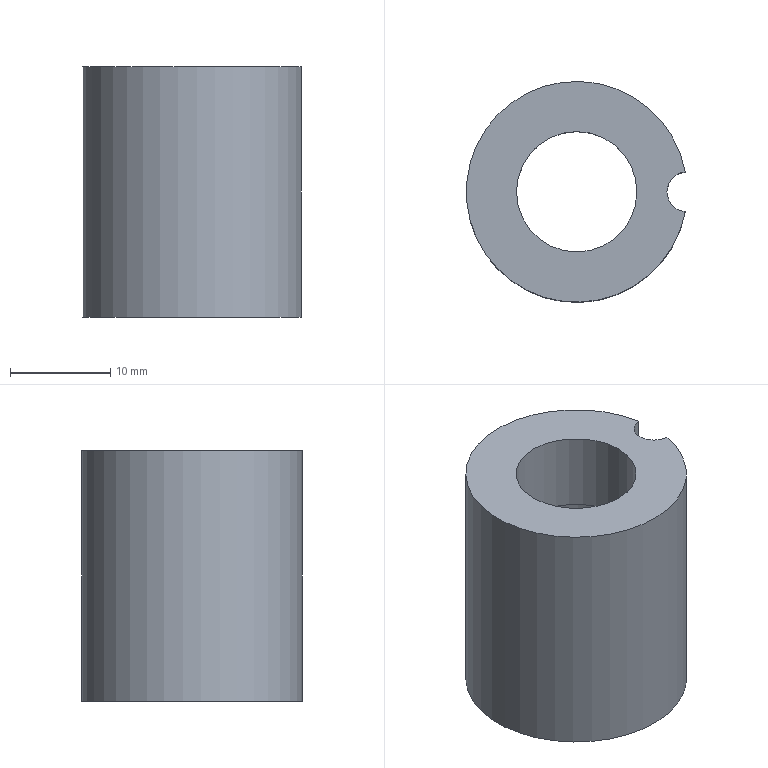Part | NX | features EKSD 22-25-12.00 2 | 1 solid | 7 faces | box 21.818 x 22 x 25 mm | volume 5601 mm3 | cylinder 4 | plane 3 | commonest cylinder face diameters 4 x1 12 x1 14.6 x1 22 x1
STEP:
#1=CARTESIAN_POINT('',(-636.682,-153.008,11.));
#2=VERTEX_POINT('',#1);
#3=CARTESIAN_POINT('',(-636.682,-156.992,11.));
#4=VERTEX_POINT('',#3);
#5=CARTESIAN_POINT('',(-636.5,-155.,11.));
#6=DIRECTION('',(0.,0.,1.));
#7=DIRECTION('',(0.,-1.,0.));
#8=AXIS2_PLACEMENT_3D('',#5,#6,#7);
#9=CIRCLE('',#8,2.);
#10=EDGE_CURVE('',#2,#4,#9,.T.);
#11=ORIENTED_EDGE('',*,*,#10,.T.);
#12=CARTESIAN_POINT('',(-647.5,-155.,11.));
#13=DIRECTION('',(0.,0.,1.));
#14=DIRECTION('',(0.,-1.,0.));
#15=AXIS2_PLACEMENT_3D('',#12,#13,#14);
#16=CIRCLE('',#15,11.);
#17=EDGE_CURVE('',#2,#4,#16,.T.);
#18=ORIENTED_EDGE('',*,*,#17,.F.);
#19=EDGE_LOOP('',(#11,#18));
#20=FACE_BOUND('',#19,.T.);
#21=CARTESIAN_POINT('',(-647.5,-147.7,11.));
#22=VERTEX_POINT('',#21);
#23=CARTESIAN_POINT('',(-647.5,-155.,11.));
#24=DIRECTION('',(0.,0.,-1.));
#25=DIRECTION('',(0.,1.,0.));
#26=AXIS2_PLACEMENT_3D('',#23,#24,#25);
#27=CIRCLE('',#26,7.3);
#28=EDGE_CURVE('',#22,#22,#27,.T.);
#29=ORIENTED_EDGE('',*,*,#28,.F.);
#30=EDGE_LOOP('',(#29));
#31=FACE_BOUND('',#30,.T.);
#32=CARTESIAN_POINT('',(-647.5,-155.,11.));
#33=DIRECTION('',(0.,0.,-1.));
#34=DIRECTION('',(0.,1.,0.));
#35=AXIS2_PLACEMENT_3D('',#32,#33,#34);
#36=PLANE('',#35);
#37=ADVANCED_FACE('',(#20,#31),#36,.T.);
#38=CARTESIAN_POINT('',(-636.682,-156.992,36.));
#39=VERTEX_POINT('',#38);
#40=CARTESIAN_POINT('',(-636.682,-153.008,36.));
#41=VERTEX_POINT('',#40);
#42=CARTESIAN_POINT('',(-636.5,-155.,36.));
#43=DIRECTION('',(0.,0.,-1.));
#44=DIRECTION('',(0.,1.,0.));
#45=AXIS2_PLACEMENT_3D('',#42,#43,#44);
#46=CIRCLE('',#45,2.);
#47=EDGE_CURVE('',#39,#41,#46,.T.);
#48=ORIENTED_EDGE('',*,*,#47,.T.);
#49=CARTESIAN_POINT('',(-647.5,-155.,36.));
#50=DIRECTION('',(0.,0.,-1.));
#51=DIRECTION('',(0.,1.,0.));
#52=AXIS2_PLACEMENT_3D('',#49,#50,#51);
#53=CIRCLE('',#52,11.);
#54=EDGE_CURVE('',#39,#41,#53,.T.);
#55=ORIENTED_EDGE('',*,*,#54,.F.);
#56=EDGE_LOOP('',(#48,#55));
#57=FACE_BOUND('',#56,.T.);
#58=CARTESIAN_POINT('',(-647.5,-161.,36.));
#59=VERTEX_POINT('',#58);
#60=CARTESIAN_POINT('',(-647.5,-155.,36.));
#61=DIRECTION('',(0.,0.,1.));
#62=DIRECTION('',(0.,-1.,0.));
#63=AXIS2_PLACEMENT_3D('',#60,#61,#62);
#64=CIRCLE('',#63,6.);
#65=EDGE_CURVE('',#59,#59,#64,.T.);
#66=ORIENTED_EDGE('',*,*,#65,.F.);
#67=EDGE_LOOP('',(#66));
#68=FACE_BOUND('',#67,.T.);
#69=CARTESIAN_POINT('',(-647.5,-155.,36.));
#70=DIRECTION('',(0.,0.,1.));
#71=DIRECTION('',(0.,-1.,0.));
#72=AXIS2_PLACEMENT_3D('',#69,#70,#71);
#73=PLANE('',#72);
#74=ADVANCED_FACE('',(#57,#68),#73,.T.);
#75=CARTESIAN_POINT('',(-636.682,-156.992,23.5));
#76=DIRECTION('',(0.,0.,-1.));
#77=VECTOR('',#76,1000.);
#78=LINE('',#75,#77);
#79=EDGE_CURVE('',#39,#4,#78,.T.);
#80=ORIENTED_EDGE('',*,*,#79,.F.);
#81=ORIENTED_EDGE('',*,*,#54,.T.);
#82=CARTESIAN_POINT('',(-636.682,-153.008,23.5));
#83=DIRECTION('',(0.,0.,-1.));
#84=VECTOR('',#83,1000.);
#85=LINE('',#82,#84);
#86=EDGE_CURVE('',#2,#41,#85,.F.);
#87=ORIENTED_EDGE('',*,*,#86,.F.);
#88=ORIENTED_EDGE('',*,*,#17,.T.);
#89=EDGE_LOOP('',(#80,#81,#87,#88));
#90=FACE_BOUND('',#89,.T.);
#91=CARTESIAN_POINT('',(-647.5,-155.,36.));
#92=DIRECTION('',(0.,0.,-1.));
#93=DIRECTION('',(0.,1.,0.));
#94=AXIS2_PLACEMENT_3D('',#91,#92,#93);
#95=CYLINDRICAL_SURFACE('',#94,11.);
#96=ADVANCED_FACE('',(#90),#95,.T.);
#97=CARTESIAN_POINT('',(-647.5,-161.,28.));
#98=VERTEX_POINT('',#97);
#99=CARTESIAN_POINT('',(-647.5,-155.,28.));
#100=DIRECTION('',(0.,0.,1.));
#101=DIRECTION('',(0.,-1.,0.));
#102=AXIS2_PLACEMENT_3D('',#99,#100,#101);
#103=CIRCLE('',#102,6.);
#104=EDGE_CURVE('',#98,#98,#103,.F.);
#105=ORIENTED_EDGE('',*,*,#104,.T.);
#106=EDGE_LOOP('',(#105));
#107=FACE_BOUND('',#106,.T.);
#108=ORIENTED_EDGE('',*,*,#65,.T.);
#109=EDGE_LOOP('',(#108));
#110=FACE_BOUND('',#109,.T.);
#111=CARTESIAN_POINT('',(-647.5,-155.,37.));
#112=DIRECTION('',(0.,0.,-1.));
#113=DIRECTION('',(0.,1.,0.));
#114=AXIS2_PLACEMENT_3D('',#111,#112,#113);
#115=CYLINDRICAL_SURFACE('',#114,6.);
#116=ADVANCED_FACE('',(#107,#110),#115,.F.);
#117=CARTESIAN_POINT('',(-647.5,-147.7,28.));
#118=VERTEX_POINT('',#117);
#119=CARTESIAN_POINT('',(-647.5,-155.,28.));
#120=DIRECTION('',(0.,0.,-1.));
#121=DIRECTION('',(0.,1.,0.));
#122=AXIS2_PLACEMENT_3D('',#119,#120,#121);
#123=CIRCLE('',#122,7.3);
#124=EDGE_CURVE('',#118,#118,#123,.T.);
#125=ORIENTED_EDGE('',*,*,#124,.T.);
#126=EDGE_LOOP('',(#125));
#127=FACE_BOUND('',#126,.T.);
#128=ORIENTED_EDGE('',*,*,#104,.F.);
#129=EDGE_LOOP('',(#128));
#130=FACE_BOUND('',#129,.T.);
#131=CARTESIAN_POINT('',(-647.5,-155.,28.));
#132=DIRECTION('',(0.,0.,1.));
#133=DIRECTION('',(0.,-1.,0.));
#134=AXIS2_PLACEMENT_3D('',#131,#132,#133);
#135=PLANE('',#134);
#136=ADVANCED_FACE('',(#127,#130),#135,.F.);
#137=ORIENTED_EDGE('',*,*,#28,.T.);
#138=EDGE_LOOP('',(#137));
#139=FACE_BOUND('',#138,.T.);
#140=ORIENTED_EDGE('',*,*,#124,.F.);
#141=EDGE_LOOP('',(#140));
#142=FACE_BOUND('',#141,.T.);
#143=CARTESIAN_POINT('',(-647.5,-155.,28.));
#144=DIRECTION('',(0.,0.,-1.));
#145=DIRECTION('',(0.,1.,0.));
#146=AXIS2_PLACEMENT_3D('',#143,#144,#145);
#147=CYLINDRICAL_SURFACE('',#146,7.3);
#148=ADVANCED_FACE('',(#139,#142),#147,.F.);
#149=ORIENTED_EDGE('',*,*,#79,.T.);
#150=ORIENTED_EDGE('',*,*,#10,.F.);
#151=ORIENTED_EDGE('',*,*,#86,.T.);
#152=ORIENTED_EDGE('',*,*,#47,.F.);
#153=EDGE_LOOP('',(#149,#150,#151,#152));
#154=FACE_BOUND('',#153,.T.);
#155=CARTESIAN_POINT('',(-636.5,-155.,36.));
#156=DIRECTION('',(0.,0.,-1.));
#157=DIRECTION('',(0.,1.,0.));
#158=AXIS2_PLACEMENT_3D('',#155,#156,#157);
#159=CYLINDRICAL_SURFACE('',#158,2.);
#160=ADVANCED_FACE('',(#154),#159,.F.);
#161=CLOSED_SHELL('',(#37,#74,#96,#116,#136,#148,#160));
#162=MANIFOLD_SOLID_BREP('',#161);
#163=(LENGTH_UNIT()NAMED_UNIT(*)SI_UNIT(.MILLI.,.METRE.));
#164=UNCERTAINTY_MEASURE_WITH_UNIT(LENGTH_MEASURE(0.00001),#163,'','');
#165=(NAMED_UNIT(*)PLANE_ANGLE_UNIT()SI_UNIT($,.RADIAN.));
#166=(NAMED_UNIT(*)SI_UNIT($,.STERADIAN.)SOLID_ANGLE_UNIT());
#167=(GEOMETRIC_REPRESENTATION_CONTEXT(3)GLOBAL_UNCERTAINTY_ASSIGNED_CONTEXT((#164))GLOBAL_UNIT_ASSIGNED_CONTEXT((#163,#165,#166))REPRESENTATION_CONTEXT('',''));
#168=ADVANCED_BREP_SHAPE_REPRESENTATION('',(#162),#167);